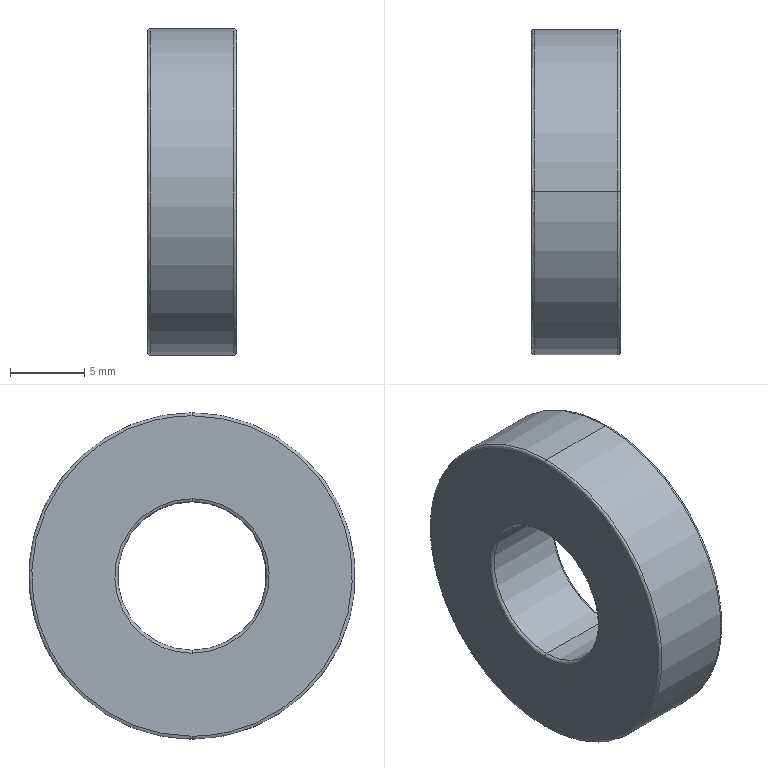Part | STEP file | Bearing B6900ZZ | 1 solid | 14 faces | box 6 x 22 x 22 mm | volume 1808 mm3 | spline 8 | cylinder 4 | plane 2 | commonest cylinder face diameters 10 x2 22 x2